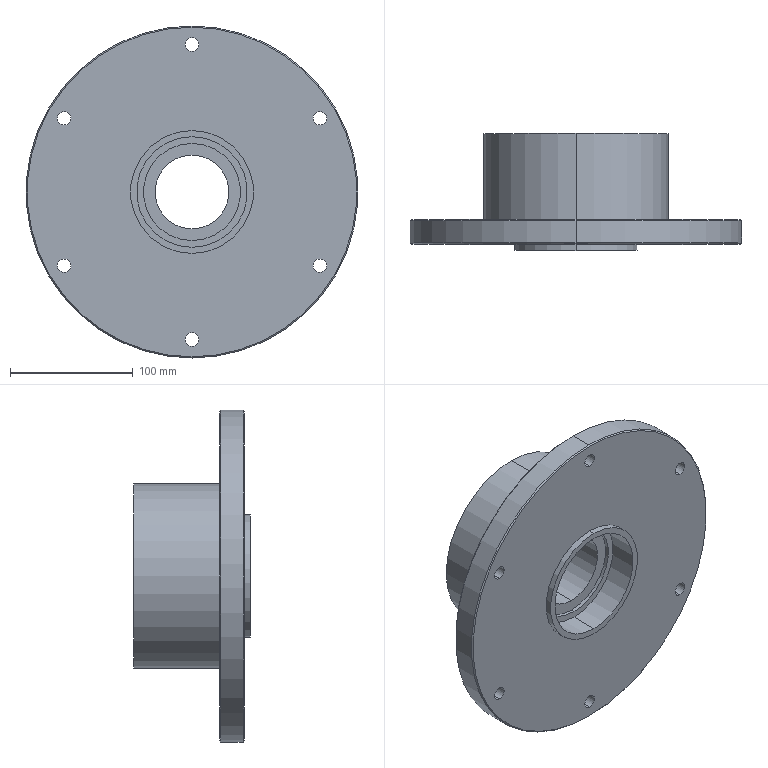Part | STEP file | BB013A02M-04-01A | 1 solid | 40 faces | box 270 x 95 x 270 mm | volume 1984635 mm3 | cylinder 28 | plane 8 | cone 4 | commonest cylinder face diameters 11 x12 79 x4 90 x4 60 x2 100 x2 150 x2